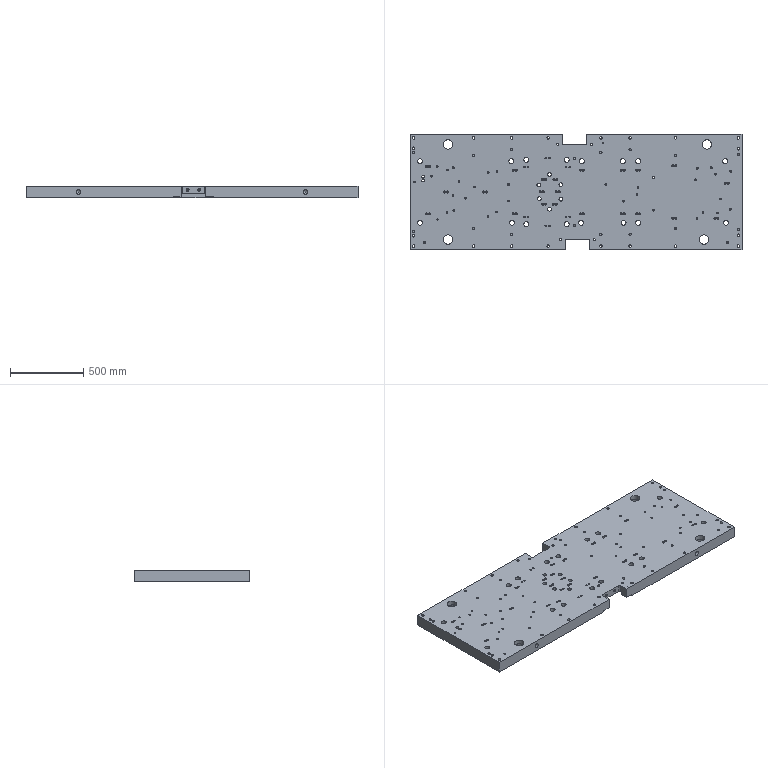Part | STEP file | 100_id66_x_t | 1 solid | 1233 faces | box 2270 x 790 x 80 mm | volume 133555884 mm3 | cylinder 623 | cone 364 | plane 246 | commonest cylinder face diameters 8.5 x126 14 x70 6.8 x67 10.3 x56 9 x44 12 x39